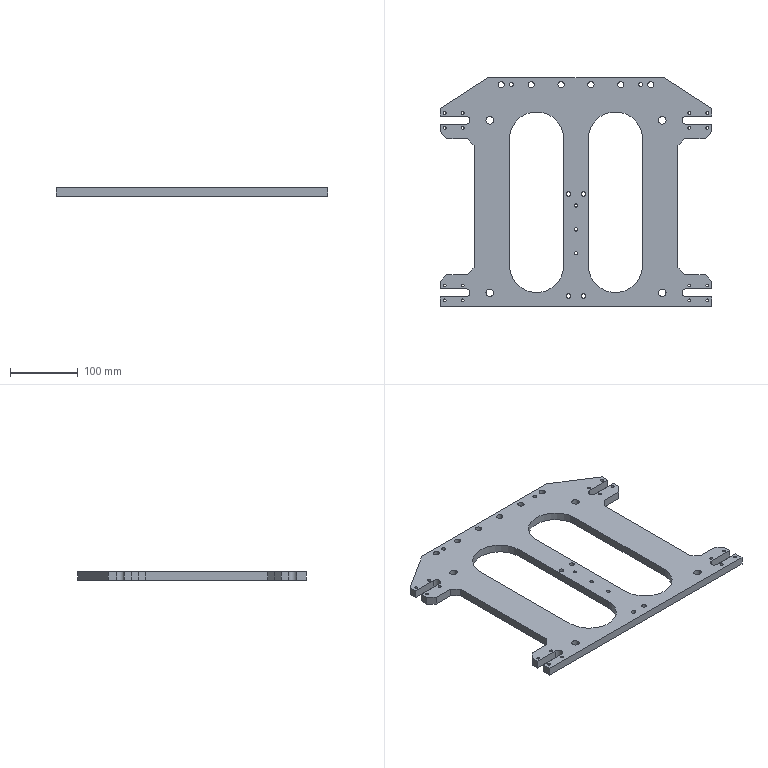NC program | NX | posted with a generic post | part box 400 x 336 x 12 mm
Lines 1 to 143 of 3199:
N10 G17 G21 G94 G90
(DRILLING , TOOL : ZXZ)
N12 T11 M6
N14 G54
N16 G17 G0 G90 X193.3 Y-159.5 S3000 M3
N18 G43 Z80. H11
N20 G94 G81 G98 Z-1. F250. R3.
N22 Y-137.5
N24 X166.7
N26 Y-159.5
N28 X127. Y-148.5
N30 X10.9 Y-3.
N32 X-10.9
N34 X0. Y-20.
N36 Y-55.
N38 Y-90.
N40 X10.9 Y-153.
N42 X-10.9
N44 X-127. Y-148.5
N46 X-166.7 Y-159.5
N48 X-193.3
N50 Y-137.5
N52 X-166.7
N54 X-193.3 Y94.5
N56 Y116.5
N58 X-166.7
N60 Y94.5
N62 X-127. Y105.5
N64 X-110. Y158.
N66 X-95.
N68 X-66.
N70 X-22.
N72 X22.
N74 X66.
N76 X95.
N78 X110.
N80 X127. Y105.5
N82 X166.7 Y116.5
N84 Y94.5
N86 X193.3
N88 Y116.5
N90 G80
N92 G0 X193.3 Y116.5 Z80.
N94 M5
(DRILLING_COPY , TOOL : 6.0ZT)
N96 T16 M6
N98 G54
N100 G17 G0 G90 X95. Y158. S2000 M3
N102 G43 Z80. H16
N104 G94 G83 G98 Z-15.303 F180. Q2. R3.
N106 X-95.
N108 G80
N110 G0 X-95. Y158. Z80.
N112 M5
(DRILLING_COPY_COPY_3 , TOOL : 5.0ZT)
N114 T15 M6
N116 G54
N118 G17 G0 G90 X0. Y-20. S2000 M3
N120 G43 Z80. H15
N122 G94 G83 G98 Z-15.002 F180. Q2. R3.
N124 Y-55.
N126 Y-90.
N128 G80
N130 G0 X0. Y-90. Z80.
N132 M5
(DRILLING_COPY_COPY_2 , TOOL : 6.6ZT)
N134 T17 M6
N136 G54
N138 G17 G0 G90 X-10.9 Y-3. S2000 M3
N140 G43 Z80. H17
N142 G94 G83 G98 Z-15.483 F180. Q2. R3.
N144 Y-153.
N146 X10.9 Y-3.
N148 Y-153.
N150 G80
N152 G0 X10.9 Y-153. Z80.
N154 M5
(DRILLING_COPY_COPY_1 , TOOL : 4.2ZT)
N156 T14 M6
N158 G54
N160 G17 G0 G90 X-166.7 Y-137.5 S2000 M3
N162 G43 Z80. H14
N164 G94 G83 G98 Z-14.762 F180. Q2. R3.
N166 Y-159.5
N168 X-193.3
N170 Y-137.5
N172 Y94.5
N174 Y116.5
N176 X-166.7
N178 Y94.5
N180 X166.7
N182 Y116.5
N184 X193.3
N186 Y94.5
N188 Y-137.5
N190 Y-159.5
N192 X166.7
N194 Y-137.5
N196 G80
N198 G0 X166.7 Y-137.5 Z80.
N200 M5
(DRILLING_COPY_COPY , TOOL : 9.0ZT)
N202 T19 M6
N204 G54
N206 G17 G0 G90 X110. Y158. S1000 M3
N208 G43 Z80. H19
N210 G94 G83 G98 Z-16.204 F180. Q2. R3.
N212 X66.
N214 X22.
N216 X-22.
N218 X-66.
N220 X-110.
N222 G80
N224 G0 X-110. Y158. Z80.
N226 M5
(DRILLING_COPY_COPY_COPY , TOOL : 11.0ZT)
N228 T12 M6
N230 G54
N232 G17 G0 G90 X127. Y105.5 S1000 M3
N234 G43 Z80. H12
N236 G94 G83 G98 Z-16.805 F180. Q2. R3.
N238 Y-148.5
N240 X-127. Y105.5
N242 Y-148.5
N244 G80
N246 G0 X-127. Y-148.5 Z80.
N248 M5